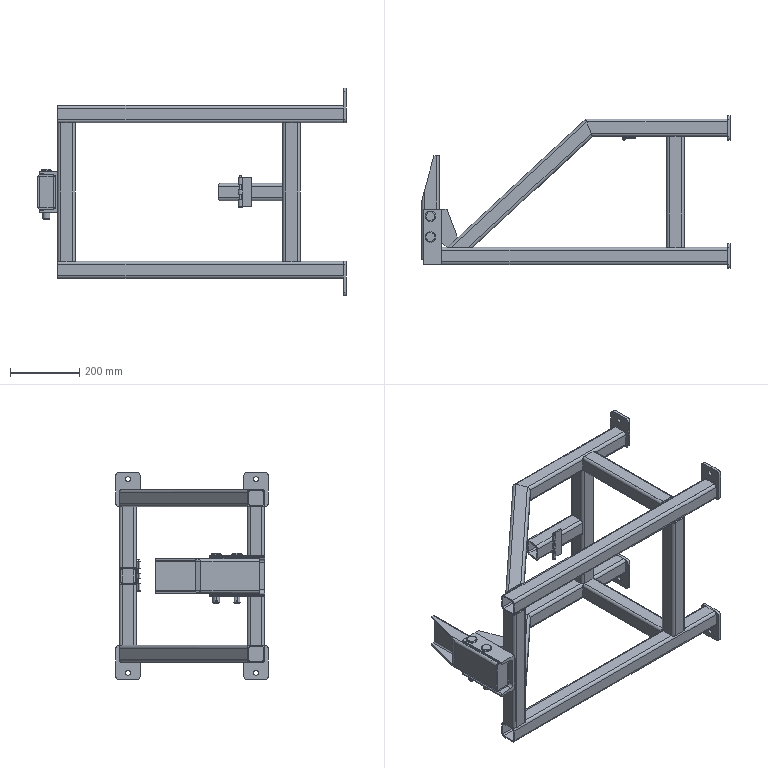Part | SolidWorks | features ReferencePattern 3, MirrorCompFeat 2 | 25 solids | 408 faces | box 891 x 440 x 600 mm | volume 4747445 mm3 | plane 211 | cylinder 183 | cone 10 | torus 4 | commonest cylinder face diameters 8 x56 16 x52 20 x28 10.5 x9 14 x8 21 x8